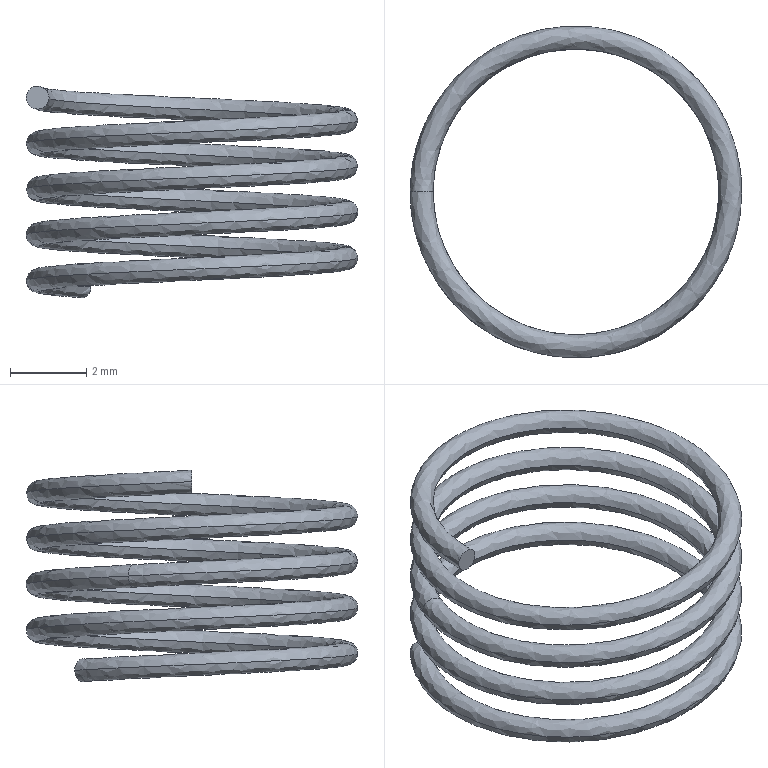Part | STEP file | ASND-0110-4216111200_SPEC_AF0 | 1 solid | 6 faces | box 8.7 x 8.7 x 5.55 mm | volume 29.663 mm3 | spline 4 | plane 2